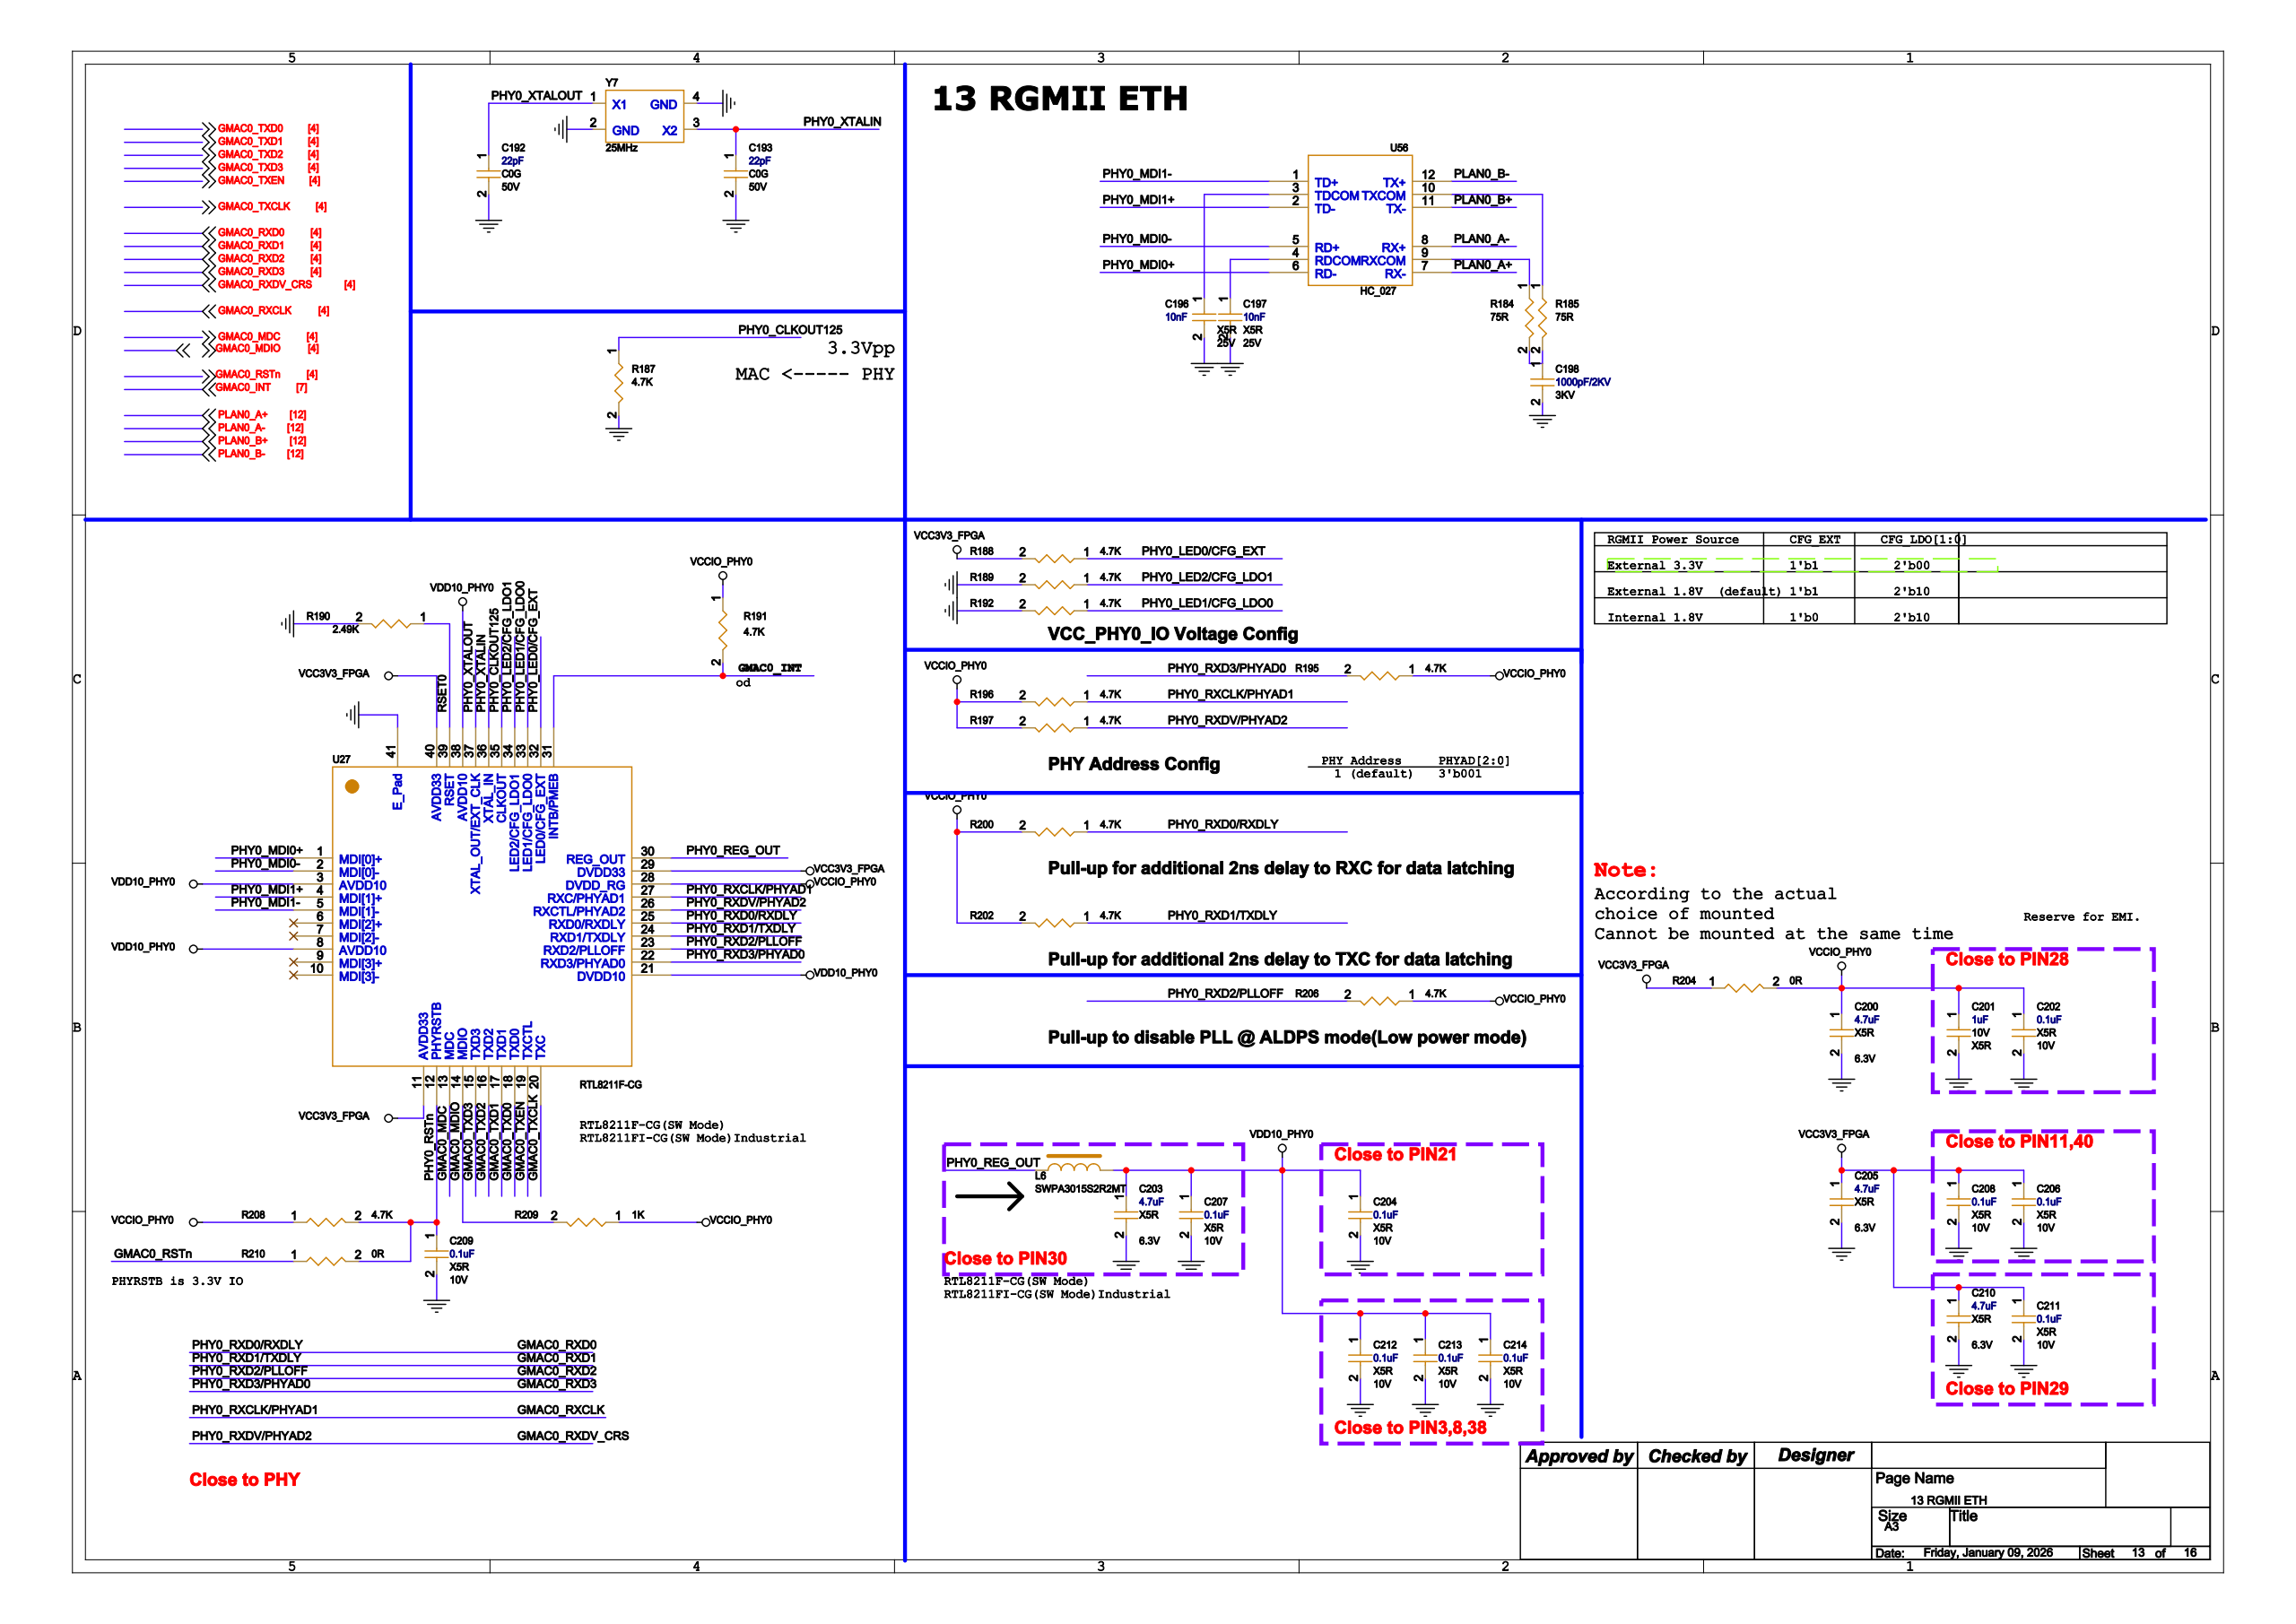Circuit board | Cadence Allegro | 442 parts | 326 nets | one sheet of the schematic
Parts on this sheet (reference | value | footprint):
C192 | 22pF | C0201
C193 | 22pF | C0201
C196 | 10nF | C0201
C197 | 10nF | C0201
C198 | 1000pF/2KV | C1206L
C200 | 4.7uF | C0402_D
C201 | 1uF | C0201
C202 | 0.1uF | C0201
C203 | 4.7uF | C0402_D
C204 | 0.1uF | C0201
C205 | 4.7uF | C0402_D
C206 | 0.1uF | C0201
C207 | 0.1uF | C0201
C208 | 0.1uF | C0201
C209 | 0.1uF | C0201
C210 | 4.7uF | C0402_D
C211 | 0.1uF | C0201
C212 | 0.1uF | C0201
C213 | 0.1uF | C0201
C214 | 0.1uF | C0201
L6 | SWPA3015S2R2MT | 1008
R184 | 75R | R0201
R185 | 75R | R0201
R187 | 4.7K | R0201
R188 | 4.7K | R0201
R189 | 4.7K | R0201
R190 | 2.49K | R0201
R191 | 4.7K | R0201
R192 | 4.7K | R0201
R195 | 4.7K | R0201
R196 | 4.7K | R0201
R197 | 4.7K | R0201
R200 | 4.7K | R0201
R202 | 4.7K | R0201
R204 | 0R | R0201
R206 | 4.7K | R0201
R208 | 4.7K | R0201
R209 | 1K | R0201
R210 | 0R | R0201
U27 | RTL8211F-CG | QFN40_5R00X5R00X0R90_T
U56 | HC_027 | HC_027
Y7 | 25MHz | OSC2520
Nets of these parts (net: part-pin ...):
GND: C192-2 C193-2 C196-2 C197-2 C198-2 C200-2 C201-2 C202-2 C203-2 C204-2 C205-2 C206-2 C207-2 C208-2 C209-2 C210-2 C211-2 C212-2 C213-2 C214-2 R187-2 R189-2 R190-2 R192-2 Y7-2 Y7-4 U27-41
PLAN0_B-: U56-12
PLAN0_B+: U56-11
PLAN0_A-: U56-8
PLAN0_A+: U56-7
VCC3V3_FPGA: C205-1 C206-1 C208-1 C210-1 C211-1 R188-2 R204-1 U27-11 U27-29 U27-40
PHY0_XTALOUT: C192-1 Y7-1 U27-37
PHY0_XTALIN: C193-1 Y7-3 U27-36
PHY0_MDI0-: U56-5 U27-2
PHY0_MDI0+: U56-6 U27-1
N49391870: C197-1 U56-4
N49391929: R184-1 U56-9
PHY0_MDI1-: U56-1 U27-5
PHY0_MDI1+: U56-2 U27-4
N49391855: C196-1 U56-3
N49391933: R185-1 U56-10
VCCIO_PHY0: C200-1 C201-1 C202-1 R191-1 R195-1 R196-2 R197-2 R200-2 R202-2 R204-2 R206-1 R208-1 R209-1 U27-28
VDD10_PHY0: C203-1 C204-1 C207-1 C212-1 C213-1 C214-1 L6-2 U27-3 U27-8 U27-21 U27-38
PHY0_RSTN: C209-1 R208-2 R210-2 U27-12
PHY0_REG_OUT: L6-1 U27-30
N17265783: C198-1 R184-2 R185-2
PHY0_CLKOUT125: R187-1 U27-35
PHY0_LED0/CFG_EXT: R188-1 U27-32
PHY0_LED2/CFG_LDO1: R189-1 U27-34
GMAC0_INT: R191-2 U27-31
PHY0_LED1/CFG_LDO0: R192-1 U27-33
GMAC0_RXD3: R195-2 U27-22
GMAC0_RXCLK: R196-1 U27-27
GMAC0_RXDV_CRS: R197-1 U27-26
GMAC0_RXD0: R200-1 U27-25
GMAC0_RXD1: R202-1 U27-24
GMAC0_RXD2: R206-2 U27-23
RSET0: R190-1 U27-39
GMAC0_RSTN: R210-1
GMAC0_MDIO: R209-2 U27-14
GMAC0_TXCLK: U27-20
GMAC0_TXD0: U27-18
GMAC0_TXD1: U27-17
GMAC0_TXD2: U27-16
GMAC0_TXD3: U27-15
GMAC0_TXEN: U27-19
GMAC0_MDC: U27-13